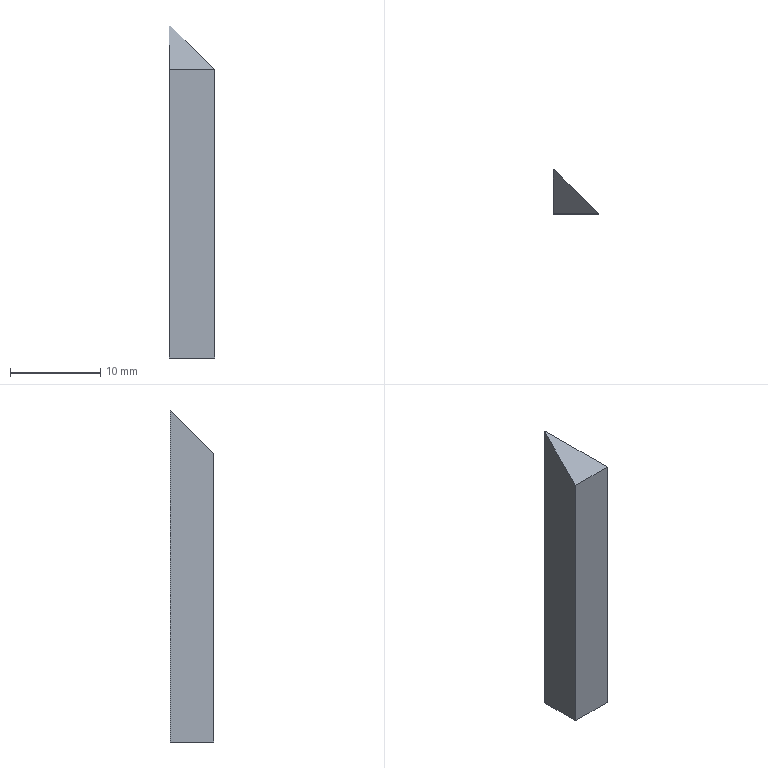Part | SolidWorks | features BaseBody 1 | 1 solid | 6 faces | box 5 x 4.859 x 36.859 mm | volume 420.464 mm3 | plane 6
STEP:
#1=CARTESIAN_POINT('',(0.1414,4.859,36.859));
#2=VERTEX_POINT('',#1);
#3=CARTESIAN_POINT('',(0.,4.859,36.859));
#4=VERTEX_POINT('',#3);
#5=CARTESIAN_POINT('',(0.,4.859,36.859));
#6=DIRECTION('',(-1.,0.,0.));
#7=VECTOR('',#6,1000.);
#8=LINE('',#5,#7);
#9=EDGE_CURVE('',#2,#4,#8,.T.);
#10=ORIENTED_EDGE('',*,*,#9,.F.);
#11=CARTESIAN_POINT('',(0.1414,4.859,0.));
#12=VERTEX_POINT('',#11);
#13=CARTESIAN_POINT('',(0.1414,4.859,37.));
#14=DIRECTION('',(0.,0.,1.));
#15=VECTOR('',#14,1000.);
#16=LINE('',#13,#15);
#17=EDGE_CURVE('',#12,#2,#16,.T.);
#18=ORIENTED_EDGE('',*,*,#17,.F.);
#19=CARTESIAN_POINT('',(0.,4.859,0.));
#20=VERTEX_POINT('',#19);
#21=CARTESIAN_POINT('',(0.,4.859,0.));
#22=DIRECTION('',(1.,0.,0.));
#23=VECTOR('',#22,1000.);
#24=LINE('',#21,#23);
#25=EDGE_CURVE('',#20,#12,#24,.T.);
#26=ORIENTED_EDGE('',*,*,#25,.F.);
#27=CARTESIAN_POINT('',(0.,4.859,37.));
#28=DIRECTION('',(0.,0.,-1.));
#29=VECTOR('',#28,1000.);
#30=LINE('',#27,#29);
#31=EDGE_CURVE('',#4,#20,#30,.T.);
#32=ORIENTED_EDGE('',*,*,#31,.F.);
#33=EDGE_LOOP('',(#10,#18,#26,#32));
#34=FACE_OUTER_BOUND('',#33,.T.);
#35=CARTESIAN_POINT('',(0.,4.859,37.));
#36=DIRECTION('',(0.,-1.,0.));
#37=DIRECTION('',(0.,0.,-1.));
#38=AXIS2_PLACEMENT_3D('',#35,#36,#37);
#39=PLANE('',#38);
#40=ADVANCED_FACE('',(#34),#39,.F.);
#41=CARTESIAN_POINT('',(5.,0.,32.));
#42=VERTEX_POINT('',#41);
#43=CARTESIAN_POINT('',(3.333,1.667,33.667));
#44=DIRECTION('',(0.5774,-0.5774,-0.5774));
#45=VECTOR('',#44,1000.);
#46=LINE('',#43,#45);
#47=EDGE_CURVE('',#2,#42,#46,.T.);
#48=ORIENTED_EDGE('',*,*,#47,.F.);
#49=ORIENTED_EDGE('',*,*,#9,.T.);
#50=CARTESIAN_POINT('',(0.,0.,32.));
#51=VERTEX_POINT('',#50);
#52=CARTESIAN_POINT('',(0.,5.,37.));
#53=DIRECTION('',(0.,-0.7071,-0.7071));
#54=VECTOR('',#53,1000.);
#55=LINE('',#52,#54);
#56=EDGE_CURVE('',#4,#51,#55,.T.);
#57=ORIENTED_EDGE('',*,*,#56,.T.);
#58=CARTESIAN_POINT('',(5.,0.,32.));
#59=DIRECTION('',(-1.,0.,0.));
#60=VECTOR('',#59,1000.);
#61=LINE('',#58,#60);
#62=EDGE_CURVE('',#42,#51,#61,.T.);
#63=ORIENTED_EDGE('',*,*,#62,.F.);
#64=EDGE_LOOP('',(#48,#49,#57,#63));
#65=FACE_OUTER_BOUND('',#64,.T.);
#66=CARTESIAN_POINT('',(5.,5.,37.));
#67=DIRECTION('',(0.,0.7071,-0.7071));
#68=DIRECTION('',(-1.,0.,0.));
#69=AXIS2_PLACEMENT_3D('',#66,#67,#68);
#70=PLANE('',#69);
#71=ADVANCED_FACE('',(#65),#70,.F.);
#72=CARTESIAN_POINT('',(0.,0.,0.));
#73=VERTEX_POINT('',#72);
#74=CARTESIAN_POINT('',(0.,0.,0.));
#75=DIRECTION('',(0.,-1.,0.));
#76=VECTOR('',#75,1000.);
#77=LINE('',#74,#76);
#78=EDGE_CURVE('',#20,#73,#77,.T.);
#79=ORIENTED_EDGE('',*,*,#78,.F.);
#80=ORIENTED_EDGE('',*,*,#25,.T.);
#81=CARTESIAN_POINT('',(5.,0.,0.));
#82=VERTEX_POINT('',#81);
#83=CARTESIAN_POINT('',(5.,0.,0.));
#84=DIRECTION('',(-0.7071,0.7071,0.));
#85=VECTOR('',#84,1000.);
#86=LINE('',#83,#85);
#87=EDGE_CURVE('',#82,#12,#86,.T.);
#88=ORIENTED_EDGE('',*,*,#87,.F.);
#89=CARTESIAN_POINT('',(0.,0.,0.));
#90=DIRECTION('',(1.,0.,0.));
#91=VECTOR('',#90,1000.);
#92=LINE('',#89,#91);
#93=EDGE_CURVE('',#73,#82,#92,.T.);
#94=ORIENTED_EDGE('',*,*,#93,.F.);
#95=EDGE_LOOP('',(#79,#80,#88,#94));
#96=FACE_OUTER_BOUND('',#95,.T.);
#97=CARTESIAN_POINT('',(0.,0.,0.));
#98=DIRECTION('',(0.,0.,1.));
#99=DIRECTION('',(1.,0.,0.));
#100=AXIS2_PLACEMENT_3D('',#97,#98,#99);
#101=PLANE('',#100);
#102=ADVANCED_FACE('',(#96),#101,.F.);
#103=ORIENTED_EDGE('',*,*,#56,.F.);
#104=ORIENTED_EDGE('',*,*,#31,.T.);
#105=ORIENTED_EDGE('',*,*,#78,.T.);
#106=CARTESIAN_POINT('',(0.,0.,37.));
#107=DIRECTION('',(0.,0.,-1.));
#108=VECTOR('',#107,1000.);
#109=LINE('',#106,#108);
#110=EDGE_CURVE('',#51,#73,#109,.T.);
#111=ORIENTED_EDGE('',*,*,#110,.F.);
#112=EDGE_LOOP('',(#103,#104,#105,#111));
#113=FACE_OUTER_BOUND('',#112,.T.);
#114=CARTESIAN_POINT('',(0.,0.,37.));
#115=DIRECTION('',(1.,0.,0.));
#116=DIRECTION('',(0.,1.,0.));
#117=AXIS2_PLACEMENT_3D('',#114,#115,#116);
#118=PLANE('',#117);
#119=ADVANCED_FACE('',(#113),#118,.F.);
#120=ORIENTED_EDGE('',*,*,#87,.T.);
#121=ORIENTED_EDGE('',*,*,#17,.T.);
#122=ORIENTED_EDGE('',*,*,#47,.T.);
#123=CARTESIAN_POINT('',(5.,0.,37.));
#124=DIRECTION('',(0.,0.,-1.));
#125=VECTOR('',#124,1000.);
#126=LINE('',#123,#125);
#127=EDGE_CURVE('',#42,#82,#126,.T.);
#128=ORIENTED_EDGE('',*,*,#127,.T.);
#129=EDGE_LOOP('',(#120,#121,#122,#128));
#130=FACE_OUTER_BOUND('',#129,.T.);
#131=CARTESIAN_POINT('',(5.,0.,37.));
#132=DIRECTION('',(-0.7071,-0.7071,0.));
#133=DIRECTION('',(-0.7071,0.7071,0.));
#134=AXIS2_PLACEMENT_3D('',#131,#132,#133);
#135=PLANE('',#134);
#136=ADVANCED_FACE('',(#130),#135,.F.);
#137=ORIENTED_EDGE('',*,*,#127,.F.);
#138=ORIENTED_EDGE('',*,*,#62,.T.);
#139=ORIENTED_EDGE('',*,*,#110,.T.);
#140=ORIENTED_EDGE('',*,*,#93,.T.);
#141=EDGE_LOOP('',(#137,#138,#139,#140));
#142=FACE_OUTER_BOUND('',#141,.T.);
#143=CARTESIAN_POINT('',(0.,0.,37.));
#144=DIRECTION('',(0.,1.,0.));
#145=DIRECTION('',(1.,0.,0.));
#146=AXIS2_PLACEMENT_3D('',#143,#144,#145);
#147=PLANE('',#146);
#148=ADVANCED_FACE('',(#142),#147,.F.);
#149=CLOSED_SHELL('',(#40,#71,#102,#119,#136,#148));
#150=MANIFOLD_SOLID_BREP('',#149);
#151=CARTESIAN_POINT('',(0.,0.,0.));
#152=DIRECTION('',(0.,0.,1.));
#153=DIRECTION('',(1.,0.,0.));
#154=AXIS2_PLACEMENT_3D('',#151,#152,#153);
#155=(LENGTH_UNIT()NAMED_UNIT(*)SI_UNIT(.MILLI.,.METRE.));
#156=UNCERTAINTY_MEASURE_WITH_UNIT(LENGTH_MEASURE(0.00001),#155,'','');
#157=(NAMED_UNIT(*)PLANE_ANGLE_UNIT()SI_UNIT($,.RADIAN.));
#158=(NAMED_UNIT(*)SI_UNIT($,.STERADIAN.)SOLID_ANGLE_UNIT());
#159=(GEOMETRIC_REPRESENTATION_CONTEXT(3)GLOBAL_UNCERTAINTY_ASSIGNED_CONTEXT((#156))GLOBAL_UNIT_ASSIGNED_CONTEXT((#155,#157,#158))REPRESENTATION_CONTEXT('',''));
#160=ADVANCED_BREP_SHAPE_REPRESENTATION('',(#150,#154),#159);